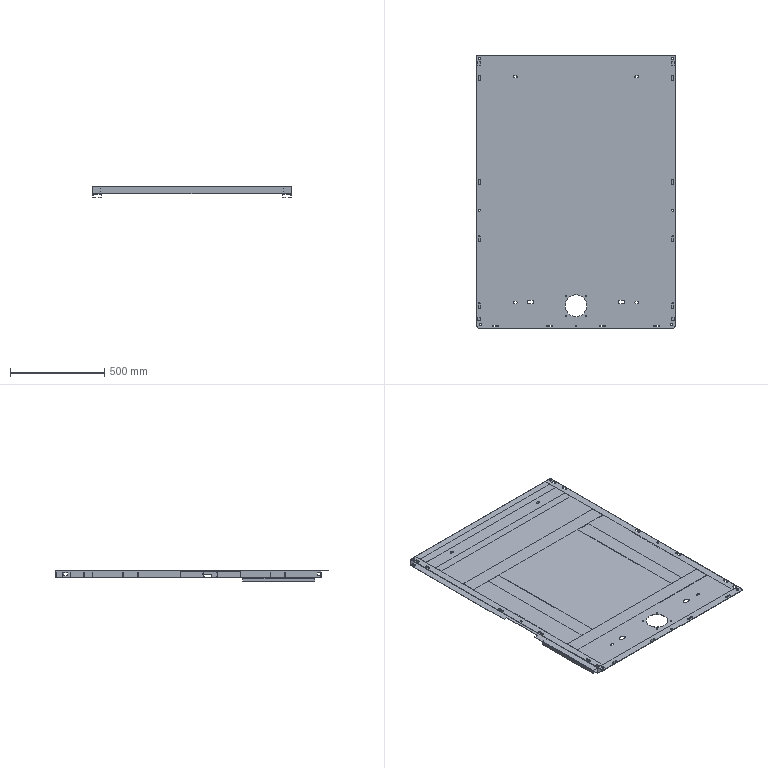Part | SolidWorks | features ReferencePattern 5, MirrorCompFeat 4, LocalLPattern 1 | 19 solids | 1132 faces | box 1050 x 1445 x 59.5 mm | volume 4576109 mm3 | plane 770 | cylinder 338 | cone 24 | commonest cylinder face diameters 10 x84 0.4 x50 3.4 x48 20 x42 11 x28 30 x10